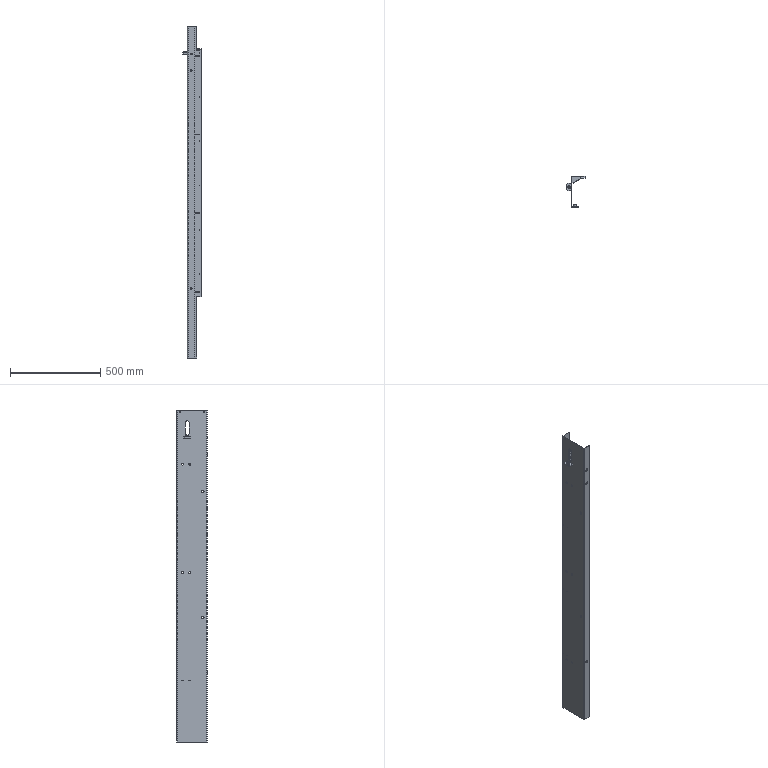Part | SolidWorks | features ICE 5, MoveCopyBody 4, Stock 4, FlatPattern 2, SMBaseFlange 2, SheetMetal 2, Chamfer 1, HoleWzd 1, LPattern 1, RefAxis 1, SMMiteredFlange 1 | 10 solids | 198 faces | box 100 x 170 x 1838 mm | volume 1271220 mm3 | plane 88 | cone 56 | cylinder 54 | commonest cylinder face diameters 10.5 x18 4.5 x12 10 x8 6 x4 13 x4 20 x3